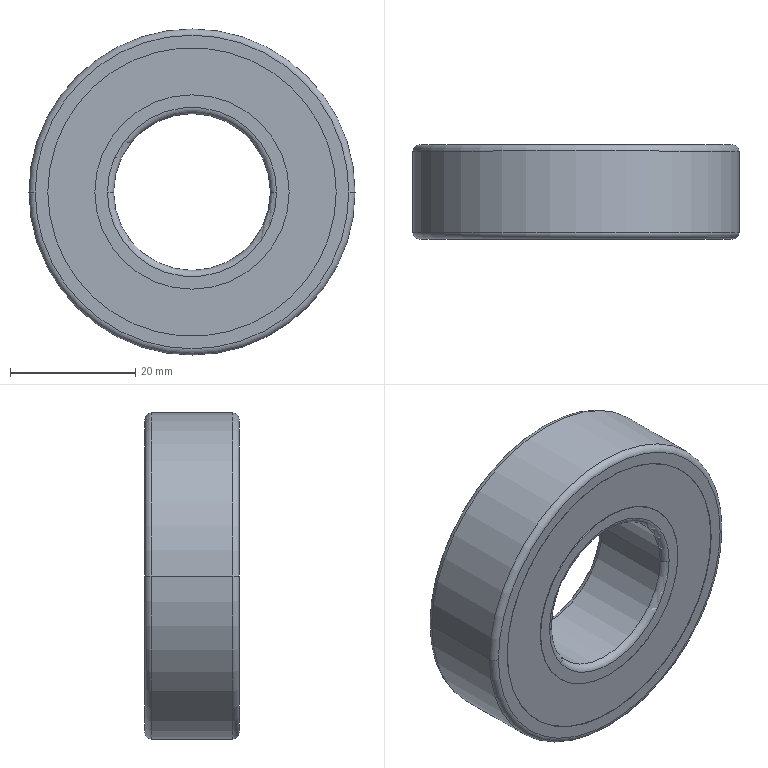Part | NX | 1 solid | 26 faces | box 52 x 15 x 52 mm | volume 24207 mm3 | cylinder 12 | torus 8 | plane 6 | commonest cylinder face diameters 31 x4 46 x4 25 x2 52 x2
STEP:
#1=CARTESIAN_POINT('',(-12.5,6.5,0.));
#2=VERTEX_POINT('',#1);
#3=CARTESIAN_POINT('',(12.5,6.5,0.));
#4=VERTEX_POINT('',#3);
#5=CARTESIAN_POINT('',(0.,6.5,0.));
#6=DIRECTION('',(0.,-1.,0.));
#7=DIRECTION('',(-1.,0.,0.));
#8=AXIS2_PLACEMENT_3D('',#5,#6,#7);
#9=CIRCLE('',#8,12.5);
#10=EDGE_CURVE('',#2,#4,#9,.T.);
#11=ORIENTED_EDGE('',*,*,#10,.T.);
#12=CARTESIAN_POINT('',(13.5,7.5,0.));
#13=VERTEX_POINT('',#12);
#14=CARTESIAN_POINT('',(13.5,6.5,0.));
#15=DIRECTION('',(0.,0.,1.));
#16=DIRECTION('',(1.,0.,0.));
#17=AXIS2_PLACEMENT_3D('',#14,#15,#16);
#18=CIRCLE('',#17,1.);
#19=EDGE_CURVE('',#13,#4,#18,.T.);
#20=ORIENTED_EDGE('',*,*,#19,.F.);
#21=CARTESIAN_POINT('',(-13.5,7.5,0.));
#22=VERTEX_POINT('',#21);
#23=CARTESIAN_POINT('',(0.,7.5,0.));
#24=DIRECTION('',(0.,1.,0.));
#25=DIRECTION('',(1.,0.,0.));
#26=AXIS2_PLACEMENT_3D('',#23,#24,#25);
#27=CIRCLE('',#26,13.5);
#28=EDGE_CURVE('',#13,#22,#27,.T.);
#29=ORIENTED_EDGE('',*,*,#28,.T.);
#30=CARTESIAN_POINT('',(-13.5,6.5,0.));
#31=DIRECTION('',(0.,0.,-1.));
#32=DIRECTION('',(-1.,0.,0.));
#33=AXIS2_PLACEMENT_3D('',#30,#31,#32);
#34=CIRCLE('',#33,1.);
#35=EDGE_CURVE('',#22,#2,#34,.T.);
#36=ORIENTED_EDGE('',*,*,#35,.T.);
#37=EDGE_LOOP('',(#11,#20,#29,#36));
#38=FACE_BOUND('',#37,.T.);
#39=CARTESIAN_POINT('',(0.,6.5,0.));
#40=DIRECTION('',(0.,-1.,0.));
#41=DIRECTION('',(-1.,0.,0.));
#42=AXIS2_PLACEMENT_3D('',#39,#40,#41);
#43=TOROIDAL_SURFACE('',#42,13.5,1.);
#44=ADVANCED_FACE('',(#38),#43,.T.);
#45=CARTESIAN_POINT('',(-15.5,7.4,0.));
#46=VERTEX_POINT('',#45);
#47=CARTESIAN_POINT('',(15.5,7.4,0.));
#48=VERTEX_POINT('',#47);
#49=CARTESIAN_POINT('',(0.,7.4,0.));
#50=DIRECTION('',(0.,1.,0.));
#51=DIRECTION('',(1.,0.,0.));
#52=AXIS2_PLACEMENT_3D('',#49,#50,#51);
#53=CIRCLE('',#52,15.5);
#54=EDGE_CURVE('',#46,#48,#53,.T.);
#55=ORIENTED_EDGE('',*,*,#54,.T.);
#56=CARTESIAN_POINT('',(15.5,7.5,0.));
#57=VERTEX_POINT('',#56);
#58=CARTESIAN_POINT('',(15.5,8.25,0.));
#59=DIRECTION('',(0.,-1.,0.));
#60=VECTOR('',#59,1000.);
#61=LINE('',#58,#60);
#62=EDGE_CURVE('',#48,#57,#61,.F.);
#63=ORIENTED_EDGE('',*,*,#62,.T.);
#64=CARTESIAN_POINT('',(-15.5,7.5,0.));
#65=VERTEX_POINT('',#64);
#66=CARTESIAN_POINT('',(0.,7.5,0.));
#67=DIRECTION('',(0.,-1.,0.));
#68=DIRECTION('',(1.,0.,0.));
#69=AXIS2_PLACEMENT_3D('',#66,#67,#68);
#70=CIRCLE('',#69,15.5);
#71=EDGE_CURVE('',#57,#65,#70,.T.);
#72=ORIENTED_EDGE('',*,*,#71,.T.);
#73=CARTESIAN_POINT('',(-15.5,8.25,0.));
#74=DIRECTION('',(0.,-1.,0.));
#75=VECTOR('',#74,1000.);
#76=LINE('',#73,#75);
#77=EDGE_CURVE('',#46,#65,#76,.F.);
#78=ORIENTED_EDGE('',*,*,#77,.F.);
#79=EDGE_LOOP('',(#55,#63,#72,#78));
#80=FACE_BOUND('',#79,.T.);
#81=CARTESIAN_POINT('',(0.,8.25,0.));
#82=DIRECTION('',(0.,-1.,0.));
#83=DIRECTION('',(-1.,0.,0.));
#84=AXIS2_PLACEMENT_3D('',#81,#82,#83);
#85=CYLINDRICAL_SURFACE('',#84,15.5);
#86=ADVANCED_FACE('',(#80),#85,.T.);
#87=CARTESIAN_POINT('',(12.5,-6.5,0.));
#88=VERTEX_POINT('',#87);
#89=CARTESIAN_POINT('',(-12.5,-6.5,0.));
#90=VERTEX_POINT('',#89);
#91=CARTESIAN_POINT('',(0.,-6.5,0.));
#92=DIRECTION('',(0.,-1.,0.));
#93=DIRECTION('',(-1.,0.,0.));
#94=AXIS2_PLACEMENT_3D('',#91,#92,#93);
#95=CIRCLE('',#94,12.5);
#96=EDGE_CURVE('',#88,#90,#95,.T.);
#97=ORIENTED_EDGE('',*,*,#96,.T.);
#98=CARTESIAN_POINT('',(-12.5,8.25,0.));
#99=DIRECTION('',(0.,-1.,0.));
#100=VECTOR('',#99,1000.);
#101=LINE('',#98,#100);
#102=EDGE_CURVE('',#90,#2,#101,.F.);
#103=ORIENTED_EDGE('',*,*,#102,.T.);
#104=CARTESIAN_POINT('',(0.,6.5,0.));
#105=DIRECTION('',(0.,-1.,0.));
#106=DIRECTION('',(-1.,0.,0.));
#107=AXIS2_PLACEMENT_3D('',#104,#105,#106);
#108=CIRCLE('',#107,12.5);
#109=EDGE_CURVE('',#4,#2,#108,.T.);
#110=ORIENTED_EDGE('',*,*,#109,.F.);
#111=CARTESIAN_POINT('',(12.5,8.25,0.));
#112=DIRECTION('',(0.,-1.,0.));
#113=VECTOR('',#112,1000.);
#114=LINE('',#111,#113);
#115=EDGE_CURVE('',#88,#4,#114,.F.);
#116=ORIENTED_EDGE('',*,*,#115,.F.);
#117=EDGE_LOOP('',(#97,#103,#110,#116));
#118=FACE_BOUND('',#117,.T.);
#119=CARTESIAN_POINT('',(0.,8.25,0.));
#120=DIRECTION('',(0.,-1.,0.));
#121=DIRECTION('',(-1.,0.,0.));
#122=AXIS2_PLACEMENT_3D('',#119,#120,#121);
#123=CYLINDRICAL_SURFACE('',#122,12.5);
#124=ADVANCED_FACE('',(#118),#123,.F.);
#125=CARTESIAN_POINT('',(-23.,7.5,0.));
#126=VERTEX_POINT('',#125);
#127=CARTESIAN_POINT('',(23.,7.5,0.));
#128=VERTEX_POINT('',#127);
#129=CARTESIAN_POINT('',(0.,7.5,0.));
#130=DIRECTION('',(0.,1.,0.));
#131=DIRECTION('',(1.,0.,0.));
#132=AXIS2_PLACEMENT_3D('',#129,#130,#131);
#133=CIRCLE('',#132,23.);
#134=EDGE_CURVE('',#126,#128,#133,.T.);
#135=ORIENTED_EDGE('',*,*,#134,.T.);
#136=CARTESIAN_POINT('',(23.,7.4,0.));
#137=VERTEX_POINT('',#136);
#138=CARTESIAN_POINT('',(23.,8.25,0.));
#139=DIRECTION('',(0.,-1.,0.));
#140=VECTOR('',#139,1000.);
#141=LINE('',#138,#140);
#142=EDGE_CURVE('',#137,#128,#141,.F.);
#143=ORIENTED_EDGE('',*,*,#142,.F.);
#144=CARTESIAN_POINT('',(-23.,7.4,0.));
#145=VERTEX_POINT('',#144);
#146=CARTESIAN_POINT('',(0.,7.4,0.));
#147=DIRECTION('',(0.,-1.,0.));
#148=DIRECTION('',(1.,0.,0.));
#149=AXIS2_PLACEMENT_3D('',#146,#147,#148);
#150=CIRCLE('',#149,23.);
#151=EDGE_CURVE('',#137,#145,#150,.T.);
#152=ORIENTED_EDGE('',*,*,#151,.T.);
#153=CARTESIAN_POINT('',(-23.,8.25,0.));
#154=DIRECTION('',(0.,-1.,0.));
#155=VECTOR('',#154,1000.);
#156=LINE('',#153,#155);
#157=EDGE_CURVE('',#145,#126,#156,.F.);
#158=ORIENTED_EDGE('',*,*,#157,.T.);
#159=EDGE_LOOP('',(#135,#143,#152,#158));
#160=FACE_BOUND('',#159,.T.);
#161=CARTESIAN_POINT('',(0.,8.25,0.));
#162=DIRECTION('',(0.,-1.,0.));
#163=DIRECTION('',(-1.,0.,0.));
#164=AXIS2_PLACEMENT_3D('',#161,#162,#163);
#165=CYLINDRICAL_SURFACE('',#164,23.);
#166=ADVANCED_FACE('',(#160),#165,.F.);
#167=ORIENTED_EDGE('',*,*,#96,.F.);
#168=CARTESIAN_POINT('',(13.5,-7.5,0.));
#169=VERTEX_POINT('',#168);
#170=CARTESIAN_POINT('',(13.5,-6.5,0.));
#171=DIRECTION('',(0.,0.,1.));
#172=DIRECTION('',(1.,0.,0.));
#173=AXIS2_PLACEMENT_3D('',#170,#171,#172);
#174=CIRCLE('',#173,1.);
#175=EDGE_CURVE('',#88,#169,#174,.T.);
#176=ORIENTED_EDGE('',*,*,#175,.T.);
#177=CARTESIAN_POINT('',(-13.5,-7.5,0.));
#178=VERTEX_POINT('',#177);
#179=CARTESIAN_POINT('',(0.,-7.5,0.));
#180=DIRECTION('',(0.,-1.,0.));
#181=DIRECTION('',(1.,0.,0.));
#182=AXIS2_PLACEMENT_3D('',#179,#180,#181);
#183=CIRCLE('',#182,13.5);
#184=EDGE_CURVE('',#169,#178,#183,.T.);
#185=ORIENTED_EDGE('',*,*,#184,.T.);
#186=CARTESIAN_POINT('',(-13.5,-6.5,0.));
#187=DIRECTION('',(0.,0.,-1.));
#188=DIRECTION('',(-1.,0.,0.));
#189=AXIS2_PLACEMENT_3D('',#186,#187,#188);
#190=CIRCLE('',#189,1.);
#191=EDGE_CURVE('',#90,#178,#190,.T.);
#192=ORIENTED_EDGE('',*,*,#191,.F.);
#193=EDGE_LOOP('',(#167,#176,#185,#192));
#194=FACE_BOUND('',#193,.T.);
#195=CARTESIAN_POINT('',(0.,-6.5,0.));
#196=DIRECTION('',(0.,-1.,0.));
#197=DIRECTION('',(-1.,0.,0.));
#198=AXIS2_PLACEMENT_3D('',#195,#196,#197);
#199=TOROIDAL_SURFACE('',#198,13.5,1.);
#200=ADVANCED_FACE('',(#194),#199,.T.);
#201=CARTESIAN_POINT('',(25.,7.5,0.));
#202=VERTEX_POINT('',#201);
#203=CARTESIAN_POINT('',(-25.,7.5,0.));
#204=VERTEX_POINT('',#203);
#205=CARTESIAN_POINT('',(0.,7.5,0.));
#206=DIRECTION('',(0.,-1.,0.));
#207=DIRECTION('',(1.,0.,0.));
#208=AXIS2_PLACEMENT_3D('',#205,#206,#207);
#209=CIRCLE('',#208,25.);
#210=EDGE_CURVE('',#202,#204,#209,.T.);
#211=ORIENTED_EDGE('',*,*,#210,.F.);
#212=CARTESIAN_POINT('',(0.,7.5,0.));
#213=DIRECTION('',(0.,-1.,0.));
#214=DIRECTION('',(1.,0.,0.));
#215=AXIS2_PLACEMENT_3D('',#212,#213,#214);
#216=CIRCLE('',#215,25.);
#217=EDGE_CURVE('',#204,#202,#216,.T.);
#218=ORIENTED_EDGE('',*,*,#217,.F.);
#219=EDGE_LOOP('',(#211,#218));
#220=FACE_BOUND('',#219,.T.);
#221=ORIENTED_EDGE('',*,*,#134,.F.);
#222=CARTESIAN_POINT('',(0.,7.5,0.));
#223=DIRECTION('',(0.,1.,0.));
#224=DIRECTION('',(1.,0.,0.));
#225=AXIS2_PLACEMENT_3D('',#222,#223,#224);
#226=CIRCLE('',#225,23.);
#227=EDGE_CURVE('',#128,#126,#226,.T.);
#228=ORIENTED_EDGE('',*,*,#227,.F.);
#229=EDGE_LOOP('',(#221,#228));
#230=FACE_BOUND('',#229,.T.);
#231=CARTESIAN_POINT('',(0.,7.5,0.));
#232=DIRECTION('',(0.,-1.,0.));
#233=DIRECTION('',(0.,0.,-1.));
#234=AXIS2_PLACEMENT_3D('',#231,#232,#233);
#235=PLANE('',#234);
#236=ADVANCED_FACE('',(#220,#230),#235,.F.);
#237=CARTESIAN_POINT('',(-15.5,-7.5,0.));
#238=VERTEX_POINT('',#237);
#239=CARTESIAN_POINT('',(15.5,-7.5,0.));
#240=VERTEX_POINT('',#239);
#241=CARTESIAN_POINT('',(0.,-7.5,0.));
#242=DIRECTION('',(0.,1.,0.));
#243=DIRECTION('',(1.,0.,0.));
#244=AXIS2_PLACEMENT_3D('',#241,#242,#243);
#245=CIRCLE('',#244,15.5);
#246=EDGE_CURVE('',#238,#240,#245,.T.);
#247=ORIENTED_EDGE('',*,*,#246,.F.);
#248=CARTESIAN_POINT('',(0.,-7.5,0.));
#249=DIRECTION('',(0.,1.,0.));
#250=DIRECTION('',(1.,0.,0.));
#251=AXIS2_PLACEMENT_3D('',#248,#249,#250);
#252=CIRCLE('',#251,15.5);
#253=EDGE_CURVE('',#240,#238,#252,.T.);
#254=ORIENTED_EDGE('',*,*,#253,.F.);
#255=EDGE_LOOP('',(#247,#254));
#256=FACE_BOUND('',#255,.T.);
#257=CARTESIAN_POINT('',(0.,-7.5,0.));
#258=DIRECTION('',(0.,-1.,0.));
#259=DIRECTION('',(1.,0.,0.));
#260=AXIS2_PLACEMENT_3D('',#257,#258,#259);
#261=CIRCLE('',#260,13.5);
#262=EDGE_CURVE('',#178,#169,#261,.T.);
#263=ORIENTED_EDGE('',*,*,#262,.F.);
#264=ORIENTED_EDGE('',*,*,#184,.F.);
#265=EDGE_LOOP('',(#263,#264));
#266=FACE_BOUND('',#265,.T.);
#267=CARTESIAN_POINT('',(0.,-7.5,0.));
#268=DIRECTION('',(0.,-1.,0.));
#269=DIRECTION('',(0.,0.,-1.));
#270=AXIS2_PLACEMENT_3D('',#267,#268,#269);
#271=PLANE('',#270);
#272=ADVANCED_FACE('',(#256,#266),#271,.T.);
#273=ORIENTED_EDGE('',*,*,#246,.T.);
#274=CARTESIAN_POINT('',(15.5,-7.4,0.));
#275=VERTEX_POINT('',#274);
#276=CARTESIAN_POINT('',(15.5,8.25,0.));
#277=DIRECTION('',(0.,-1.,0.));
#278=VECTOR('',#277,1000.);
#279=LINE('',#276,#278);
#280=EDGE_CURVE('',#240,#275,#279,.F.);
#281=ORIENTED_EDGE('',*,*,#280,.T.);
#282=CARTESIAN_POINT('',(-15.5,-7.4,0.));
#283=VERTEX_POINT('',#282);
#284=CARTESIAN_POINT('',(0.,-7.4,0.));
#285=DIRECTION('',(0.,-1.,0.));
#286=DIRECTION('',(1.,0.,0.));
#287=AXIS2_PLACEMENT_3D('',#284,#285,#286);
#288=CIRCLE('',#287,15.5);
#289=EDGE_CURVE('',#275,#283,#288,.T.);
#290=ORIENTED_EDGE('',*,*,#289,.T.);
#291=CARTESIAN_POINT('',(-15.5,8.25,0.));
#292=DIRECTION('',(0.,-1.,0.));
#293=VECTOR('',#292,1000.);
#294=LINE('',#291,#293);
#295=EDGE_CURVE('',#238,#283,#294,.F.);
#296=ORIENTED_EDGE('',*,*,#295,.F.);
#297=EDGE_LOOP('',(#273,#281,#290,#296));
#298=FACE_BOUND('',#297,.T.);
#299=CARTESIAN_POINT('',(0.,8.25,0.));
#300=DIRECTION('',(0.,-1.,0.));
#301=DIRECTION('',(-1.,0.,0.));
#302=AXIS2_PLACEMENT_3D('',#299,#300,#301);
#303=CYLINDRICAL_SURFACE('',#302,15.5);
#304=ADVANCED_FACE('',(#298),#303,.T.);
#305=CARTESIAN_POINT('',(-26.,6.5,0.));
#306=VERTEX_POINT('',#305);
#307=CARTESIAN_POINT('',(26.,6.5,0.));
#308=VERTEX_POINT('',#307);
#309=CARTESIAN_POINT('',(0.,6.5,0.));
#310=DIRECTION('',(0.,-1.,0.));
#311=DIRECTION('',(-1.,0.,0.));
#312=AXIS2_PLACEMENT_3D('',#309,#310,#311);
#313=CIRCLE('',#312,26.);
#314=EDGE_CURVE('',#306,#308,#313,.T.);
#315=ORIENTED_EDGE('',*,*,#314,.F.);
#316=CARTESIAN_POINT('',(-25.,6.5,0.));
#317=DIRECTION('',(0.,0.,-1.));
#318=DIRECTION('',(-1.,0.,0.));
#319=AXIS2_PLACEMENT_3D('',#316,#317,#318);
#320=CIRCLE('',#319,1.);
#321=EDGE_CURVE('',#204,#306,#320,.F.);
#322=ORIENTED_EDGE('',*,*,#321,.F.);
#323=ORIENTED_EDGE('',*,*,#217,.T.);
#324=CARTESIAN_POINT('',(25.,6.5,0.));
#325=DIRECTION('',(0.,0.,1.));
#326=DIRECTION('',(1.,0.,0.));
#327=AXIS2_PLACEMENT_3D('',#324,#325,#326);
#328=CIRCLE('',#327,1.);
#329=EDGE_CURVE('',#202,#308,#328,.F.);
#330=ORIENTED_EDGE('',*,*,#329,.T.);
#331=EDGE_LOOP('',(#315,#322,#323,#330));
#332=FACE_BOUND('',#331,.T.);
#333=CARTESIAN_POINT('',(0.,6.5,0.));
#334=DIRECTION('',(0.,-1.,0.));
#335=DIRECTION('',(-1.,0.,0.));
#336=AXIS2_PLACEMENT_3D('',#333,#334,#335);
#337=TOROIDAL_SURFACE('',#336,25.,1.);
#338=ADVANCED_FACE('',(#332),#337,.T.);
#339=CARTESIAN_POINT('',(23.,-7.4,0.));
#340=VERTEX_POINT('',#339);
#341=CARTESIAN_POINT('',(-23.,-7.4,0.));
#342=VERTEX_POINT('',#341);
#343=CARTESIAN_POINT('',(0.,-7.4,0.));
#344=DIRECTION('',(0.,1.,0.));
#345=DIRECTION('',(1.,0.,0.));
#346=AXIS2_PLACEMENT_3D('',#343,#344,#345);
#347=CIRCLE('',#346,23.);
#348=EDGE_CURVE('',#340,#342,#347,.T.);
#349=ORIENTED_EDGE('',*,*,#348,.F.);
#350=CARTESIAN_POINT('',(0.,-7.4,0.));
#351=DIRECTION('',(0.,1.,0.));
#352=DIRECTION('',(1.,0.,0.));
#353=AXIS2_PLACEMENT_3D('',#350,#351,#352);
#354=CIRCLE('',#353,23.);
#355=EDGE_CURVE('',#342,#340,#354,.T.);
#356=ORIENTED_EDGE('',*,*,#355,.F.);
#357=EDGE_LOOP('',(#349,#356));
#358=FACE_BOUND('',#357,.T.);
#359=ORIENTED_EDGE('',*,*,#289,.F.);
#360=CARTESIAN_POINT('',(0.,-7.4,0.));
#361=DIRECTION('',(0.,-1.,0.));
#362=DIRECTION('',(1.,0.,0.));
#363=AXIS2_PLACEMENT_3D('',#360,#361,#362);
#364=CIRCLE('',#363,15.5);
#365=EDGE_CURVE('',#283,#275,#364,.T.);
#366=ORIENTED_EDGE('',*,*,#365,.F.);
#367=EDGE_LOOP('',(#359,#366));
#368=FACE_BOUND('',#367,.T.);
#369=CARTESIAN_POINT('',(0.,-7.4,0.));
#370=DIRECTION('',(0.,-1.,0.));
#371=DIRECTION('',(0.,0.,-1.));
#372=AXIS2_PLACEMENT_3D('',#369,#370,#371);
#373=PLANE('',#372);
#374=ADVANCED_FACE('',(#358,#368),#373,.T.);
#375=CARTESIAN_POINT('',(-23.,-7.5,0.));
#376=VERTEX_POINT('',#375);
#377=CARTESIAN_POINT('',(23.,-7.5,0.));
#378=VERTEX_POINT('',#377);
#379=CARTESIAN_POINT('',(0.,-7.5,0.));
#380=DIRECTION('',(0.,-1.,0.));
#381=DIRECTION('',(1.,0.,0.));
#382=AXIS2_PLACEMENT_3D('',#379,#380,#381);
#383=CIRCLE('',#382,23.);
#384=EDGE_CURVE('',#376,#378,#383,.T.);
#385=ORIENTED_EDGE('',*,*,#384,.T.);
#386=CARTESIAN_POINT('',(23.,8.25,0.));
#387=DIRECTION('',(0.,-1.,0.));
#388=VECTOR('',#387,1000.);
#389=LINE('',#386,#388);
#390=EDGE_CURVE('',#378,#340,#389,.F.);
#391=ORIENTED_EDGE('',*,*,#390,.T.);
#392=ORIENTED_EDGE('',*,*,#348,.T.);
#393=CARTESIAN_POINT('',(-23.,8.25,0.));
#394=DIRECTION('',(0.,-1.,0.));
#395=VECTOR('',#394,1000.);
#396=LINE('',#393,#395);
#397=EDGE_CURVE('',#376,#342,#396,.F.);
#398=ORIENTED_EDGE('',*,*,#397,.F.);
#399=EDGE_LOOP('',(#385,#391,#392,#398));
#400=FACE_BOUND('',#399,.T.);
#401=CARTESIAN_POINT('',(0.,8.25,0.));
#402=DIRECTION('',(0.,-1.,0.));
#403=DIRECTION('',(-1.,0.,0.));
#404=AXIS2_PLACEMENT_3D('',#401,#402,#403);
#405=CYLINDRICAL_SURFACE('',#404,23.);
#406=ADVANCED_FACE('',(#400),#405,.F.);
#407=ORIENTED_EDGE('',*,*,#151,.F.);
#408=CARTESIAN_POINT('',(0.,7.4,0.));
#409=DIRECTION('',(0.,-1.,0.));
#410=DIRECTION('',(1.,0.,0.));
#411=AXIS2_PLACEMENT_3D('',#408,#409,#410);
#412=CIRCLE('',#411,23.);
#413=EDGE_CURVE('',#145,#137,#412,.T.);
#414=ORIENTED_EDGE('',*,*,#413,.F.);
#415=EDGE_LOOP('',(#407,#414));
#416=FACE_BOUND('',#415,.T.);
#417=ORIENTED_EDGE('',*,*,#54,.F.);
#418=CARTESIAN_POINT('',(0.,7.4,0.));
#419=DIRECTION('',(0.,1.,0.));
#420=DIRECTION('',(1.,0.,0.));
#421=AXIS2_PLACEMENT_3D('',#418,#419,#420);
#422=CIRCLE('',#421,15.5);
#423=EDGE_CURVE('',#48,#46,#422,.T.);
#424=ORIENTED_EDGE('',*,*,#423,.F.);
#425=EDGE_LOOP('',(#417,#424));
#426=FACE_BOUND('',#425,.T.);
#427=CARTESIAN_POINT('',(0.,7.4,0.));
#428=DIRECTION('',(0.,-1.,0.));
#429=DIRECTION('',(0.,0.,-1.));
#430=AXIS2_PLACEMENT_3D('',#427,#428,#429);
#431=PLANE('',#430);
#432=ADVANCED_FACE('',(#416,#426),#431,.F.);
#433=CARTESIAN_POINT('',(25.,-7.5,0.));
#434=VERTEX_POINT('',#433);
#435=CARTESIAN_POINT('',(-25.,-7.5,0.));
#436=VERTEX_POINT('',#435);
#437=CARTESIAN_POINT('',(0.,-7.5,0.));
#438=DIRECTION('',(0.,1.,0.));
#439=DIRECTION('',(1.,0.,0.));
#440=AXIS2_PLACEMENT_3D('',#437,#438,#439);
#441=CIRCLE('',#440,25.);
#442=EDGE_CURVE('',#434,#436,#441,.T.);
#443=ORIENTED_EDGE('',*,*,#442,.F.);
#444=CARTESIAN_POINT('',(0.,-7.5,0.));
#445=DIRECTION('',(0.,1.,0.));
#446=DIRECTION('',(1.,0.,0.));
#447=AXIS2_PLACEMENT_3D('',#444,#445,#446);
#448=CIRCLE('',#447,25.);
#449=EDGE_CURVE('',#436,#434,#448,.T.);
#450=ORIENTED_EDGE('',*,*,#449,.F.);
#451=EDGE_LOOP('',(#443,#450));
#452=FACE_BOUND('',#451,.T.);
#453=ORIENTED_EDGE('',*,*,#384,.F.);
#454=CARTESIAN_POINT('',(0.,-7.5,0.));
#455=DIRECTION('',(0.,-1.,0.));
#456=DIRECTION('',(1.,0.,0.));
#457=AXIS2_PLACEMENT_3D('',#454,#455,#456);
#458=CIRCLE('',#457,23.);
#459=EDGE_CURVE('',#378,#376,#458,.T.);
#460=ORIENTED_EDGE('',*,*,#459,.F.);
#461=EDGE_LOOP('',(#453,#460));
#462=FACE_BOUND('',#461,.T.);
#463=CARTESIAN_POINT('',(0.,-7.5,0.));
#464=DIRECTION('',(0.,-1.,0.));
#465=DIRECTION('',(0.,0.,-1.));
#466=AXIS2_PLACEMENT_3D('',#463,#464,#465);
#467=PLANE('',#466);
#468=ADVANCED_FACE('',(#452,#462),#467,.T.);
#469=ORIENTED_EDGE('',*,*,#442,.T.);
#470=CARTESIAN_POINT('',(-26.,-6.5,0.));
#471=VERTEX_POINT('',#470);
#472=CARTESIAN_POINT('',(-25.,-6.5,0.));
#473=DIRECTION('',(0.,0.,-1.));
#474=DIRECTION('',(-1.,0.,0.));
#475=AXIS2_PLACEMENT_3D('',#472,#473,#474);
#476=CIRCLE('',#475,1.);
#477=EDGE_CURVE('',#471,#436,#476,.F.);
#478=ORIENTED_EDGE('',*,*,#477,.F.);
#479=CARTESIAN_POINT('',(26.,-6.5,0.));
#480=VERTEX_POINT('',#479);
#481=CARTESIAN_POINT('',(0.,-6.5,0.));
#482=DIRECTION('',(0.,-1.,0.));
#483=DIRECTION('',(-1.,0.,0.));
#484=AXIS2_PLACEMENT_3D('',#481,#482,#483);
#485=CIRCLE('',#484,26.);
#486=EDGE_CURVE('',#471,#480,#485,.T.);
#487=ORIENTED_EDGE('',*,*,#486,.T.);
#488=CARTESIAN_POINT('',(25.,-6.5,0.));
#489=DIRECTION('',(0.,0.,1.));
#490=DIRECTION('',(1.,0.,0.));
#491=AXIS2_PLACEMENT_3D('',#488,#489,#490);
#492=CIRCLE('',#491,1.);
#493=EDGE_CURVE('',#480,#434,#492,.F.);
#494=ORIENTED_EDGE('',*,*,#493,.T.);
#495=EDGE_LOOP('',(#469,#478,#487,#494));
#496=FACE_BOUND('',#495,.T.);
#497=CARTESIAN_POINT('',(0.,-6.5,0.));
#498=DIRECTION('',(0.,-1.,0.));
#499=DIRECTION('',(-1.,0.,0.));
#500=AXIS2_PLACEMENT_3D('',#497,#498,#499);
#501=TOROIDAL_SURFACE('',#500,25.,1.);
#502=ADVANCED_FACE('',(#496),#501,.T.);
#503=ORIENTED_EDGE('',*,*,#71,.F.);
#504=CARTESIAN_POINT('',(0.,7.5,0.));
#505=DIRECTION('',(0.,-1.,0.));
#506=DIRECTION('',(1.,0.,0.));
#507=AXIS2_PLACEMENT_3D('',#504,#505,#506);
#508=CIRCLE('',#507,15.5);
#509=EDGE_CURVE('',#65,#57,#508,.T.);
#510=ORIENTED_EDGE('',*,*,#509,.F.);
#511=EDGE_LOOP('',(#503,#510));
#512=FACE_BOUND('',#511,.T.);
#513=CARTESIAN_POINT('',(0.,7.5,0.));
#514=DIRECTION('',(0.,1.,0.));
#515=DIRECTION('',(1.,0.,0.));
#516=AXIS2_PLACEMENT_3D('',#513,#514,#515);
#517=CIRCLE('',#516,13.5);
#518=EDGE_CURVE('',#22,#13,#517,.T.);
#519=ORIENTED_EDGE('',*,*,#518,.F.);
#520=ORIENTED_EDGE('',*,*,#28,.F.);
#521=EDGE_LOOP('',(#519,#520));
#522=FACE_BOUND('',#521,.T.);
#523=CARTESIAN_POINT('',(0.,7.5,0.));
#524=DIRECTION('',(0.,-1.,0.));
#525=DIRECTION('',(0.,0.,-1.));
#526=AXIS2_PLACEMENT_3D('',#523,#524,#525);
#527=PLANE('',#526);
#528=ADVANCED_FACE('',(#512,#522),#527,.F.);
#529=CARTESIAN_POINT('',(0.,-6.5,0.));
#530=DIRECTION('',(0.,-1.,0.));
#531=DIRECTION('',(-1.,0.,0.));
#532=AXIS2_PLACEMENT_3D('',#529,#530,#531);
#533=CIRCLE('',#532,26.);
#534=EDGE_CURVE('',#480,#471,#533,.T.);
#535=ORIENTED_EDGE('',*,*,#534,.F.);
#536=CARTESIAN_POINT('',(26.,8.25,0.));
#537=DIRECTION('',(0.,-1.,0.));
#538=VECTOR('',#537,1000.);
#539=LINE('',#536,#538);
#540=EDGE_CURVE('',#308,#480,#539,.T.);
#541=ORIENTED_EDGE('',*,*,#540,.F.);
#542=CARTESIAN_POINT('',(0.,6.5,0.));
#543=DIRECTION('',(0.,-1.,0.));
#544=DIRECTION('',(-1.,0.,0.));
#545=AXIS2_PLACEMENT_3D('',#542,#543,#544);
#546=CIRCLE('',#545,26.);
#547=EDGE_CURVE('',#308,#306,#546,.T.);
#548=ORIENTED_EDGE('',*,*,#547,.T.);
#549=CARTESIAN_POINT('',(-26.,8.25,0.));
#550=DIRECTION('',(0.,-1.,0.));
#551=VECTOR('',#550,1000.);
#552=LINE('',#549,#551);
#553=EDGE_CURVE('',#306,#471,#552,.T.);
#554=ORIENTED_EDGE('',*,*,#553,.T.);
#555=EDGE_LOOP('',(#535,#541,#548,#554));
#556=FACE_BOUND('',#555,.T.);
#557=CARTESIAN_POINT('',(0.,8.25,0.));
#558=DIRECTION('',(0.,-1.,0.));
#559=DIRECTION('',(-1.,0.,0.));
#560=AXIS2_PLACEMENT_3D('',#557,#558,#559);
#561=CYLINDRICAL_SURFACE('',#560,26.);
#562=ADVANCED_FACE('',(#556),#561,.T.);
#563=ORIENTED_EDGE('',*,*,#295,.T.);
#564=ORIENTED_EDGE('',*,*,#365,.T.);
#565=ORIENTED_EDGE('',*,*,#280,.F.);
#566=ORIENTED_EDGE('',*,*,#253,.T.);
#567=EDGE_LOOP('',(#563,#564,#565,#566));
#568=FACE_BOUND('',#567,.T.);
#569=CARTESIAN_POINT('',(0.,8.25,0.));
#570=DIRECTION('',(0.,-1.,0.));
#571=DIRECTION('',(-1.,0.,0.));
#572=AXIS2_PLACEMENT_3D('',#569,#570,#571);
#573=CYLINDRICAL_SURFACE('',#572,15.5);
#574=ADVANCED_FACE('',(#568),#573,.T.);
#575=ORIENTED_EDGE('',*,*,#10,.F.);
#576=ORIENTED_EDGE('',*,*,#102,.F.);
#577=CARTESIAN_POINT('',(0.,-6.5,0.));
#578=DIRECTION('',(0.,-1.,0.));
#579=DIRECTION('',(-1.,0.,0.));
#580=AXIS2_PLACEMENT_3D('',#577,#578,#579);
#581=CIRCLE('',#580,12.5);
#582=EDGE_CURVE('',#90,#88,#581,.T.);
#583=ORIENTED_EDGE('',*,*,#582,.T.);
#584=ORIENTED_EDGE('',*,*,#115,.T.);
#585=EDGE_LOOP('',(#575,#576,#583,#584));
#586=FACE_BOUND('',#585,.T.);
#587=CARTESIAN_POINT('',(0.,8.25,0.));
#588=DIRECTION('',(0.,-1.,0.));
#589=DIRECTION('',(-1.,0.,0.));
#590=AXIS2_PLACEMENT_3D('',#587,#588,#589);
#591=CYLINDRICAL_SURFACE('',#590,12.5);
#592=ADVANCED_FACE('',(#586),#591,.F.);
#593=ORIENTED_EDGE('',*,*,#77,.T.);
#594=ORIENTED_EDGE('',*,*,#509,.T.);
#595=ORIENTED_EDGE('',*,*,#62,.F.);
#596=ORIENTED_EDGE('',*,*,#423,.T.);
#597=EDGE_LOOP('',(#593,#594,#595,#596));
#598=FACE_BOUND('',#597,.T.);
#599=CARTESIAN_POINT('',(0.,8.25,0.));
#600=DIRECTION('',(0.,-1.,0.));
#601=DIRECTION('',(-1.,0.,0.));
#602=AXIS2_PLACEMENT_3D('',#599,#600,#601);
#603=CYLINDRICAL_SURFACE('',#602,15.5);
#604=ADVANCED_FACE('',(#598),#603,.T.);
#605=ORIENTED_EDGE('',*,*,#157,.F.);
#606=ORIENTED_EDGE('',*,*,#413,.T.);
#607=ORIENTED_EDGE('',*,*,#142,.T.);
#608=ORIENTED_EDGE('',*,*,#227,.T.);
#609=EDGE_LOOP('',(#605,#606,#607,#608));
#610=FACE_BOUND('',#609,.T.);
#611=CARTESIAN_POINT('',(0.,8.25,0.));
#612=DIRECTION('',(0.,-1.,0.));
#613=DIRECTION('',(-1.,0.,0.));
#614=AXIS2_PLACEMENT_3D('',#611,#612,#613);
#615=CYLINDRICAL_SURFACE('',#614,23.);
#616=ADVANCED_FACE('',(#610),#615,.F.);
#617=ORIENTED_EDGE('',*,*,#314,.T.);
#618=ORIENTED_EDGE('',*,*,#540,.T.);
#619=ORIENTED_EDGE('',*,*,#486,.F.);
#620=ORIENTED_EDGE('',*,*,#553,.F.);
#621=EDGE_LOOP('',(#617,#618,#619,#620));
#622=FACE_BOUND('',#621,.T.);
#623=CARTESIAN_POINT('',(0.,8.25,0.));
#624=DIRECTION('',(0.,-1.,0.));
#625=DIRECTION('',(-1.,0.,0.));
#626=AXIS2_PLACEMENT_3D('',#623,#624,#625);
#627=CYLINDRICAL_SURFACE('',#626,26.);
#628=ADVANCED_FACE('',(#622),#627,.T.);
#629=ORIENTED_EDGE('',*,*,#397,.T.);
#630=ORIENTED_EDGE('',*,*,#355,.T.);
#631=ORIENTED_EDGE('',*,*,#390,.F.);
#632=ORIENTED_EDGE('',*,*,#459,.T.);
#633=EDGE_LOOP('',(#629,#630,#631,#632));
#634=FACE_BOUND('',#633,.T.);
#635=CARTESIAN_POINT('',(0.,8.25,0.));
#636=DIRECTION('',(0.,-1.,0.));
#637=DIRECTION('',(-1.,0.,0.));
#638=AXIS2_PLACEMENT_3D('',#635,#636,#637);
#639=CYLINDRICAL_SURFACE('',#638,23.);
#640=ADVANCED_FACE('',(#634),#639,.F.);
#641=ORIENTED_EDGE('',*,*,#210,.T.);
#642=ORIENTED_EDGE('',*,*,#321,.T.);
#643=ORIENTED_EDGE('',*,*,#547,.F.);
#644=ORIENTED_EDGE('',*,*,#329,.F.);
#645=EDGE_LOOP('',(#641,#642,#643,#644));
#646=FACE_BOUND('',#645,.T.);
#647=CARTESIAN_POINT('',(0.,6.5,0.));
#648=DIRECTION('',(0.,-1.,0.));
#649=DIRECTION('',(-1.,0.,0.));
#650=AXIS2_PLACEMENT_3D('',#647,#648,#649);
#651=TOROIDAL_SURFACE('',#650,25.,1.);
#652=ADVANCED_FACE('',(#646),#651,.T.);
#653=ORIENTED_EDGE('',*,*,#262,.T.);
#654=ORIENTED_EDGE('',*,*,#175,.F.);
#655=ORIENTED_EDGE('',*,*,#582,.F.);
#656=ORIENTED_EDGE('',*,*,#191,.T.);
#657=EDGE_LOOP('',(#653,#654,#655,#656));
#658=FACE_BOUND('',#657,.T.);
#659=CARTESIAN_POINT('',(0.,-6.5,0.));
#660=DIRECTION('',(0.,-1.,0.));
#661=DIRECTION('',(-1.,0.,0.));
#662=AXIS2_PLACEMENT_3D('',#659,#660,#661);
#663=TOROIDAL_SURFACE('',#662,13.5,1.);
#664=ADVANCED_FACE('',(#658),#663,.T.);
#665=ORIENTED_EDGE('',*,*,#534,.T.);
#666=ORIENTED_EDGE('',*,*,#477,.T.);
#667=ORIENTED_EDGE('',*,*,#449,.T.);
#668=ORIENTED_EDGE('',*,*,#493,.F.);
#669=EDGE_LOOP('',(#665,#666,#667,#668));
#670=FACE_BOUND('',#669,.T.);
#671=CARTESIAN_POINT('',(0.,-6.5,0.));
#672=DIRECTION('',(0.,-1.,0.));
#673=DIRECTION('',(-1.,0.,0.));
#674=AXIS2_PLACEMENT_3D('',#671,#672,#673);
#675=TOROIDAL_SURFACE('',#674,25.,1.);
#676=ADVANCED_FACE('',(#670),#675,.T.);
#677=ORIENTED_EDGE('',*,*,#518,.T.);
#678=ORIENTED_EDGE('',*,*,#19,.T.);
#679=ORIENTED_EDGE('',*,*,#109,.T.);
#680=ORIENTED_EDGE('',*,*,#35,.F.);
#681=EDGE_LOOP('',(#677,#678,#679,#680));
#682=FACE_BOUND('',#681,.T.);
#683=CARTESIAN_POINT('',(0.,6.5,0.));
#684=DIRECTION('',(0.,-1.,0.));
#685=DIRECTION('',(-1.,0.,0.));
#686=AXIS2_PLACEMENT_3D('',#683,#684,#685);
#687=TOROIDAL_SURFACE('',#686,13.5,1.);
#688=ADVANCED_FACE('',(#682),#687,.T.);
#689=CLOSED_SHELL('',(#44,#86,#124,#166,#200,#236,#272,#304,#338,#374,#406,#432,#468,#502,#528,#562,#574,#592,#604,#616,#628,#640,#652,#664,#676,#688));
#690=MANIFOLD_SOLID_BREP('',#689);
#691=(LENGTH_UNIT()NAMED_UNIT(*)SI_UNIT(.MILLI.,.METRE.));
#692=UNCERTAINTY_MEASURE_WITH_UNIT(LENGTH_MEASURE(0.00001),#691,'','');
#693=(NAMED_UNIT(*)PLANE_ANGLE_UNIT()SI_UNIT($,.RADIAN.));
#694=(NAMED_UNIT(*)SI_UNIT($,.STERADIAN.)SOLID_ANGLE_UNIT());
#695=(GEOMETRIC_REPRESENTATION_CONTEXT(3)GLOBAL_UNCERTAINTY_ASSIGNED_CONTEXT((#692))GLOBAL_UNIT_ASSIGNED_CONTEXT((#691,#693,#694))REPRESENTATION_CONTEXT('',''));
#696=ADVANCED_BREP_SHAPE_REPRESENTATION('',(#690),#695);